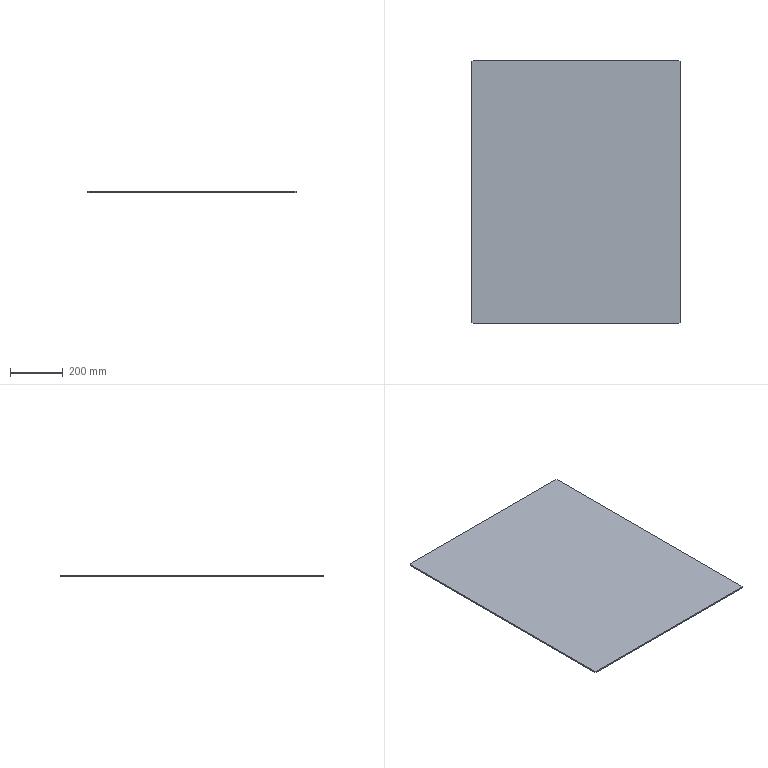Part | SolidWorks | features Chamfer 1, Extrusion 1 | 1 solid | 10 faces | box 790 x 1000 x 5 mm | volume 3949750 mm3 | plane 10
STEP:
#1=CARTESIAN_POINT('',(-395.,495.,0.));
#2=VERTEX_POINT('',#1);
#3=CARTESIAN_POINT('',(-395.,-495.,0.));
#4=VERTEX_POINT('',#3);
#5=CARTESIAN_POINT('',(-395.,500.,0.));
#6=DIRECTION('',(0.,-1.,0.));
#7=VECTOR('',#6,1000.);
#8=LINE('',#5,#7);
#9=EDGE_CURVE('',#2,#4,#8,.T.);
#10=ORIENTED_EDGE('',*,*,#9,.T.);
#11=CARTESIAN_POINT('',(-395.,-495.,5.));
#12=VERTEX_POINT('',#11);
#13=CARTESIAN_POINT('',(-395.,-495.,5.));
#14=DIRECTION('',(0.,0.,1.));
#15=VECTOR('',#14,1000.);
#16=LINE('',#13,#15);
#17=EDGE_CURVE('',#4,#12,#16,.T.);
#18=ORIENTED_EDGE('',*,*,#17,.T.);
#19=CARTESIAN_POINT('',(-395.,495.,5.));
#20=VERTEX_POINT('',#19);
#21=CARTESIAN_POINT('',(-395.,500.,5.));
#22=DIRECTION('',(0.,-1.,0.));
#23=VECTOR('',#22,1000.);
#24=LINE('',#21,#23);
#25=EDGE_CURVE('',#20,#12,#24,.T.);
#26=ORIENTED_EDGE('',*,*,#25,.F.);
#27=CARTESIAN_POINT('',(-395.,495.,5.));
#28=DIRECTION('',(0.,0.,-1.));
#29=VECTOR('',#28,1000.);
#30=LINE('',#27,#29);
#31=EDGE_CURVE('',#20,#2,#30,.T.);
#32=ORIENTED_EDGE('',*,*,#31,.T.);
#33=EDGE_LOOP('',(#10,#18,#26,#32));
#34=FACE_OUTER_BOUND('',#33,.T.);
#35=CARTESIAN_POINT('',(-395.,500.,5.));
#36=DIRECTION('',(1.,0.,0.));
#37=DIRECTION('',(0.,1.,0.));
#38=AXIS2_PLACEMENT_3D('',#35,#36,#37);
#39=PLANE('',#38);
#40=ADVANCED_FACE('',(#34),#39,.F.);
#41=CARTESIAN_POINT('',(-390.,-500.,5.));
#42=VERTEX_POINT('',#41);
#43=CARTESIAN_POINT('',(390.,-500.,5.));
#44=VERTEX_POINT('',#43);
#45=CARTESIAN_POINT('',(-395.,-500.,5.));
#46=DIRECTION('',(1.,0.,0.));
#47=VECTOR('',#46,1000.);
#48=LINE('',#45,#47);
#49=EDGE_CURVE('',#42,#44,#48,.T.);
#50=ORIENTED_EDGE('',*,*,#49,.F.);
#51=CARTESIAN_POINT('',(-390.,-500.,0.));
#52=VERTEX_POINT('',#51);
#53=CARTESIAN_POINT('',(-390.,-500.,5.));
#54=DIRECTION('',(0.,0.,-1.));
#55=VECTOR('',#54,1000.);
#56=LINE('',#53,#55);
#57=EDGE_CURVE('',#42,#52,#56,.T.);
#58=ORIENTED_EDGE('',*,*,#57,.T.);
#59=CARTESIAN_POINT('',(390.,-500.,0.));
#60=VERTEX_POINT('',#59);
#61=CARTESIAN_POINT('',(-395.,-500.,0.));
#62=DIRECTION('',(1.,0.,0.));
#63=VECTOR('',#62,1000.);
#64=LINE('',#61,#63);
#65=EDGE_CURVE('',#52,#60,#64,.T.);
#66=ORIENTED_EDGE('',*,*,#65,.T.);
#67=CARTESIAN_POINT('',(390.,-500.,5.));
#68=DIRECTION('',(0.,0.,1.));
#69=VECTOR('',#68,1000.);
#70=LINE('',#67,#69);
#71=EDGE_CURVE('',#60,#44,#70,.T.);
#72=ORIENTED_EDGE('',*,*,#71,.T.);
#73=EDGE_LOOP('',(#50,#58,#66,#72));
#74=FACE_OUTER_BOUND('',#73,.T.);
#75=CARTESIAN_POINT('',(-395.,-500.,5.));
#76=DIRECTION('',(0.,1.,0.));
#77=DIRECTION('',(0.,0.,1.));
#78=AXIS2_PLACEMENT_3D('',#75,#76,#77);
#79=PLANE('',#78);
#80=ADVANCED_FACE('',(#74),#79,.F.);
#81=CARTESIAN_POINT('',(395.,-495.,5.));
#82=VERTEX_POINT('',#81);
#83=CARTESIAN_POINT('',(395.,495.,5.));
#84=VERTEX_POINT('',#83);
#85=CARTESIAN_POINT('',(395.,500.,5.));
#86=DIRECTION('',(0.,1.,0.));
#87=VECTOR('',#86,1000.);
#88=LINE('',#85,#87);
#89=EDGE_CURVE('',#82,#84,#88,.T.);
#90=ORIENTED_EDGE('',*,*,#89,.F.);
#91=CARTESIAN_POINT('',(395.,-495.,0.));
#92=VERTEX_POINT('',#91);
#93=CARTESIAN_POINT('',(395.,-495.,5.));
#94=DIRECTION('',(0.,0.,-1.));
#95=VECTOR('',#94,1000.);
#96=LINE('',#93,#95);
#97=EDGE_CURVE('',#82,#92,#96,.T.);
#98=ORIENTED_EDGE('',*,*,#97,.T.);
#99=CARTESIAN_POINT('',(395.,495.,0.));
#100=VERTEX_POINT('',#99);
#101=CARTESIAN_POINT('',(395.,500.,0.));
#102=DIRECTION('',(0.,1.,0.));
#103=VECTOR('',#102,1000.);
#104=LINE('',#101,#103);
#105=EDGE_CURVE('',#92,#100,#104,.T.);
#106=ORIENTED_EDGE('',*,*,#105,.T.);
#107=CARTESIAN_POINT('',(395.,495.,5.));
#108=DIRECTION('',(0.,0.,1.));
#109=VECTOR('',#108,1000.);
#110=LINE('',#107,#109);
#111=EDGE_CURVE('',#100,#84,#110,.T.);
#112=ORIENTED_EDGE('',*,*,#111,.T.);
#113=EDGE_LOOP('',(#90,#98,#106,#112));
#114=FACE_OUTER_BOUND('',#113,.T.);
#115=CARTESIAN_POINT('',(395.,500.,5.));
#116=DIRECTION('',(-1.,0.,0.));
#117=DIRECTION('',(0.,-1.,0.));
#118=AXIS2_PLACEMENT_3D('',#115,#116,#117);
#119=PLANE('',#118);
#120=ADVANCED_FACE('',(#114),#119,.F.);
#121=CARTESIAN_POINT('',(390.,500.,5.));
#122=VERTEX_POINT('',#121);
#123=CARTESIAN_POINT('',(-390.,500.,5.));
#124=VERTEX_POINT('',#123);
#125=CARTESIAN_POINT('',(-395.,500.,5.));
#126=DIRECTION('',(-1.,0.,0.));
#127=VECTOR('',#126,1000.);
#128=LINE('',#125,#127);
#129=EDGE_CURVE('',#122,#124,#128,.T.);
#130=ORIENTED_EDGE('',*,*,#129,.F.);
#131=CARTESIAN_POINT('',(390.,500.,0.));
#132=VERTEX_POINT('',#131);
#133=CARTESIAN_POINT('',(390.,500.,5.));
#134=DIRECTION('',(0.,0.,-1.));
#135=VECTOR('',#134,1000.);
#136=LINE('',#133,#135);
#137=EDGE_CURVE('',#122,#132,#136,.T.);
#138=ORIENTED_EDGE('',*,*,#137,.T.);
#139=CARTESIAN_POINT('',(-390.,500.,0.));
#140=VERTEX_POINT('',#139);
#141=CARTESIAN_POINT('',(-395.,500.,0.));
#142=DIRECTION('',(-1.,0.,0.));
#143=VECTOR('',#142,1000.);
#144=LINE('',#141,#143);
#145=EDGE_CURVE('',#132,#140,#144,.T.);
#146=ORIENTED_EDGE('',*,*,#145,.T.);
#147=CARTESIAN_POINT('',(-390.,500.,5.));
#148=DIRECTION('',(0.,0.,1.));
#149=VECTOR('',#148,1000.);
#150=LINE('',#147,#149);
#151=EDGE_CURVE('',#140,#124,#150,.T.);
#152=ORIENTED_EDGE('',*,*,#151,.T.);
#153=EDGE_LOOP('',(#130,#138,#146,#152));
#154=FACE_OUTER_BOUND('',#153,.T.);
#155=CARTESIAN_POINT('',(-395.,500.,5.));
#156=DIRECTION('',(0.,-1.,0.));
#157=DIRECTION('',(0.,0.,-1.));
#158=AXIS2_PLACEMENT_3D('',#155,#156,#157);
#159=PLANE('',#158);
#160=ADVANCED_FACE('',(#154),#159,.F.);
#161=ORIENTED_EDGE('',*,*,#25,.T.);
#162=CARTESIAN_POINT('',(-392.5,-497.5,5.));
#163=DIRECTION('',(0.7071,-0.7071,0.));
#164=VECTOR('',#163,1000.);
#165=LINE('',#162,#164);
#166=EDGE_CURVE('',#12,#42,#165,.T.);
#167=ORIENTED_EDGE('',*,*,#166,.T.);
#168=ORIENTED_EDGE('',*,*,#49,.T.);
#169=CARTESIAN_POINT('',(-2.5,-892.5,5.));
#170=DIRECTION('',(0.7071,0.7071,0.));
#171=VECTOR('',#170,1000.);
#172=LINE('',#169,#171);
#173=EDGE_CURVE('',#44,#82,#172,.T.);
#174=ORIENTED_EDGE('',*,*,#173,.T.);
#175=ORIENTED_EDGE('',*,*,#89,.T.);
#176=CARTESIAN_POINT('',(497.5,392.5,5.));
#177=DIRECTION('',(-0.7071,0.7071,0.));
#178=VECTOR('',#177,1000.);
#179=LINE('',#176,#178);
#180=EDGE_CURVE('',#84,#122,#179,.T.);
#181=ORIENTED_EDGE('',*,*,#180,.T.);
#182=ORIENTED_EDGE('',*,*,#129,.T.);
#183=CARTESIAN_POINT('',(-892.5,-2.5,5.));
#184=DIRECTION('',(-0.7071,-0.7071,0.));
#185=VECTOR('',#184,1000.);
#186=LINE('',#183,#185);
#187=EDGE_CURVE('',#124,#20,#186,.T.);
#188=ORIENTED_EDGE('',*,*,#187,.T.);
#189=EDGE_LOOP('',(#161,#167,#168,#174,#175,#181,#182,#188));
#190=FACE_OUTER_BOUND('',#189,.T.);
#191=CARTESIAN_POINT('',(-395.,-500.,5.));
#192=DIRECTION('',(0.,0.,1.));
#193=DIRECTION('',(1.,0.,0.));
#194=AXIS2_PLACEMENT_3D('',#191,#192,#193);
#195=PLANE('',#194);
#196=ADVANCED_FACE('',(#190),#195,.T.);
#197=ORIENTED_EDGE('',*,*,#65,.F.);
#198=CARTESIAN_POINT('',(-390.,-500.,0.));
#199=DIRECTION('',(-0.7071,0.7071,0.));
#200=VECTOR('',#199,1000.);
#201=LINE('',#198,#200);
#202=EDGE_CURVE('',#52,#4,#201,.T.);
#203=ORIENTED_EDGE('',*,*,#202,.T.);
#204=ORIENTED_EDGE('',*,*,#9,.F.);
#205=CARTESIAN_POINT('',(-395.,495.,0.));
#206=DIRECTION('',(0.7071,0.7071,0.));
#207=VECTOR('',#206,1000.);
#208=LINE('',#205,#207);
#209=EDGE_CURVE('',#2,#140,#208,.T.);
#210=ORIENTED_EDGE('',*,*,#209,.T.);
#211=ORIENTED_EDGE('',*,*,#145,.F.);
#212=CARTESIAN_POINT('',(390.,500.,0.));
#213=DIRECTION('',(0.7071,-0.7071,0.));
#214=VECTOR('',#213,1000.);
#215=LINE('',#212,#214);
#216=EDGE_CURVE('',#132,#100,#215,.T.);
#217=ORIENTED_EDGE('',*,*,#216,.T.);
#218=ORIENTED_EDGE('',*,*,#105,.F.);
#219=CARTESIAN_POINT('',(395.,-495.,0.));
#220=DIRECTION('',(-0.7071,-0.7071,0.));
#221=VECTOR('',#220,1000.);
#222=LINE('',#219,#221);
#223=EDGE_CURVE('',#92,#60,#222,.T.);
#224=ORIENTED_EDGE('',*,*,#223,.T.);
#225=EDGE_LOOP('',(#197,#203,#204,#210,#211,#217,#218,#224));
#226=FACE_OUTER_BOUND('',#225,.T.);
#227=CARTESIAN_POINT('',(-395.,-500.,0.));
#228=DIRECTION('',(0.,0.,1.));
#229=DIRECTION('',(1.,0.,0.));
#230=AXIS2_PLACEMENT_3D('',#227,#228,#229);
#231=PLANE('',#230);
#232=ADVANCED_FACE('',(#226),#231,.F.);
#233=ORIENTED_EDGE('',*,*,#166,.F.);
#234=ORIENTED_EDGE('',*,*,#17,.F.);
#235=ORIENTED_EDGE('',*,*,#202,.F.);
#236=ORIENTED_EDGE('',*,*,#57,.F.);
#237=EDGE_LOOP('',(#233,#234,#235,#236));
#238=FACE_OUTER_BOUND('',#237,.T.);
#239=CARTESIAN_POINT('',(-390.,-500.,5.));
#240=DIRECTION('',(0.7071,0.7071,0.));
#241=DIRECTION('',(-0.7071,0.7071,0.));
#242=AXIS2_PLACEMENT_3D('',#239,#240,#241);
#243=PLANE('',#242);
#244=ADVANCED_FACE('',(#238),#243,.F.);
#245=ORIENTED_EDGE('',*,*,#173,.F.);
#246=ORIENTED_EDGE('',*,*,#71,.F.);
#247=ORIENTED_EDGE('',*,*,#223,.F.);
#248=ORIENTED_EDGE('',*,*,#97,.F.);
#249=EDGE_LOOP('',(#245,#246,#247,#248));
#250=FACE_OUTER_BOUND('',#249,.T.);
#251=CARTESIAN_POINT('',(395.,-495.,5.));
#252=DIRECTION('',(-0.7071,0.7071,0.));
#253=DIRECTION('',(-0.7071,-0.7071,0.));
#254=AXIS2_PLACEMENT_3D('',#251,#252,#253);
#255=PLANE('',#254);
#256=ADVANCED_FACE('',(#250),#255,.F.);
#257=ORIENTED_EDGE('',*,*,#180,.F.);
#258=ORIENTED_EDGE('',*,*,#111,.F.);
#259=ORIENTED_EDGE('',*,*,#216,.F.);
#260=ORIENTED_EDGE('',*,*,#137,.F.);
#261=EDGE_LOOP('',(#257,#258,#259,#260));
#262=FACE_OUTER_BOUND('',#261,.T.);
#263=CARTESIAN_POINT('',(390.,500.,5.));
#264=DIRECTION('',(-0.7071,-0.7071,0.));
#265=DIRECTION('',(0.7071,-0.7071,0.));
#266=AXIS2_PLACEMENT_3D('',#263,#264,#265);
#267=PLANE('',#266);
#268=ADVANCED_FACE('',(#262),#267,.F.);
#269=ORIENTED_EDGE('',*,*,#187,.F.);
#270=ORIENTED_EDGE('',*,*,#151,.F.);
#271=ORIENTED_EDGE('',*,*,#209,.F.);
#272=ORIENTED_EDGE('',*,*,#31,.F.);
#273=EDGE_LOOP('',(#269,#270,#271,#272));
#274=FACE_OUTER_BOUND('',#273,.T.);
#275=CARTESIAN_POINT('',(-395.,495.,5.));
#276=DIRECTION('',(0.7071,-0.7071,0.));
#277=DIRECTION('',(0.7071,0.7071,0.));
#278=AXIS2_PLACEMENT_3D('',#275,#276,#277);
#279=PLANE('',#278);
#280=ADVANCED_FACE('',(#274),#279,.F.);
#281=CLOSED_SHELL('',(#40,#80,#120,#160,#196,#232,#244,#256,#268,#280));
#282=MANIFOLD_SOLID_BREP('',#281);
#283=CARTESIAN_POINT('',(0.,0.,0.));
#284=DIRECTION('',(0.,0.,1.));
#285=DIRECTION('',(1.,0.,0.));
#286=AXIS2_PLACEMENT_3D('',#283,#284,#285);
#287=(LENGTH_UNIT()NAMED_UNIT(*)SI_UNIT(.MILLI.,.METRE.));
#288=UNCERTAINTY_MEASURE_WITH_UNIT(LENGTH_MEASURE(0.00001),#287,'','');
#289=(NAMED_UNIT(*)PLANE_ANGLE_UNIT()SI_UNIT($,.RADIAN.));
#290=(NAMED_UNIT(*)SI_UNIT($,.STERADIAN.)SOLID_ANGLE_UNIT());
#291=(GEOMETRIC_REPRESENTATION_CONTEXT(3)GLOBAL_UNCERTAINTY_ASSIGNED_CONTEXT((#288))GLOBAL_UNIT_ASSIGNED_CONTEXT((#287,#289,#290))REPRESENTATION_CONTEXT('',''));
#292=ADVANCED_BREP_SHAPE_REPRESENTATION('',(#282,#286),#291);